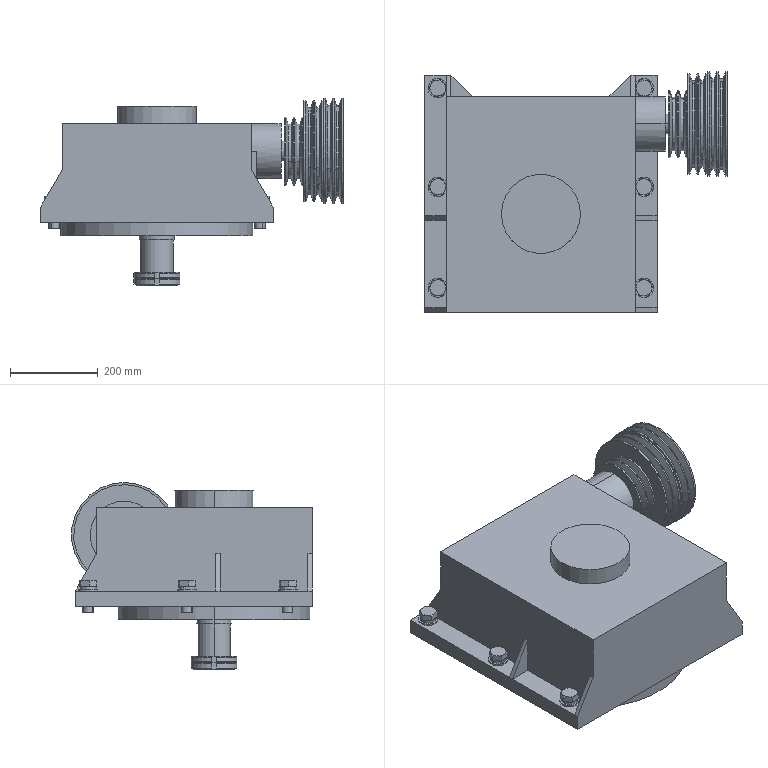Part | SolidWorks | features ReferencePattern 3, MirrorCompFeat 1 | 23 solids | 491 faces | box 690 x 549 x 426.5 mm | volume 59127815 mm3 | plane 182 | cylinder 161 | cone 124 | torus 24 | commonest cylinder face diameters 24.5 x18 36.439 x18 24 x12 25 x12 30 x12 44 x12